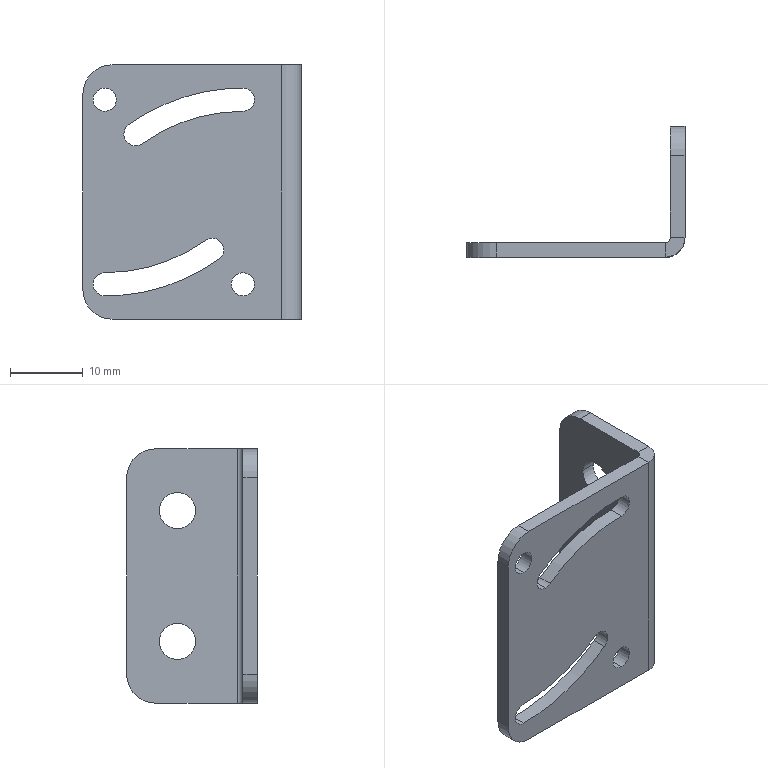Part | STEP file | KF-2212-070-006 | 1 solid | 35 faces | box 30 x 18 x 35 mm | volume 2796 mm3 | cylinder 23 | plane 12 | commonest cylinder face diameters 3.2 x9 5 x4 8 x4 47.6 x2 54 x2 1.473 x1
STEP:
#1=CARTESIAN_POINT('',(30.,6.5,-26.5));
#2=VERTEX_POINT('',#1);
#3=CARTESIAN_POINT('',(30.,11.5,-26.5));
#4=VERTEX_POINT('',#3);
#5=CARTESIAN_POINT('',(30.,9.,-26.5));
#6=DIRECTION('',(1.,0.,0.));
#7=DIRECTION('',(0.,-1.,0.));
#8=AXIS2_PLACEMENT_3D('',#5,#6,#7);
#9=CIRCLE('',#8,2.5);
#10=EDGE_CURVE('',#2,#4,#9,.T.);
#11=ORIENTED_EDGE('',*,*,#10,.T.);
#12=CARTESIAN_POINT('',(28.,11.5,-26.5));
#13=VERTEX_POINT('',#12);
#14=CARTESIAN_POINT('',(38.,11.5,-26.5));
#15=DIRECTION('',(-1.,0.,0.));
#16=VECTOR('',#15,1000.);
#17=LINE('',#14,#16);
#18=EDGE_CURVE('',#4,#13,#17,.T.);
#19=ORIENTED_EDGE('',*,*,#18,.T.);
#20=CARTESIAN_POINT('',(28.,6.5,-26.5));
#21=VERTEX_POINT('',#20);
#22=CARTESIAN_POINT('',(28.,9.,-26.5));
#23=DIRECTION('',(1.,0.,0.));
#24=DIRECTION('',(0.,-1.,0.));
#25=AXIS2_PLACEMENT_3D('',#22,#23,#24);
#26=CIRCLE('',#25,2.5);
#27=EDGE_CURVE('',#21,#13,#26,.T.);
#28=ORIENTED_EDGE('',*,*,#27,.F.);
#29=CARTESIAN_POINT('',(38.,6.5,-26.5));
#30=DIRECTION('',(-1.,0.,0.));
#31=VECTOR('',#30,1000.);
#32=LINE('',#29,#31);
#33=EDGE_CURVE('',#2,#21,#32,.T.);
#34=ORIENTED_EDGE('',*,*,#33,.F.);
#35=EDGE_LOOP('',(#11,#19,#28,#34));
#36=FACE_OUTER_BOUND('',#35,.T.);
#37=CARTESIAN_POINT('',(38.,9.,-26.5));
#38=DIRECTION('',(-1.,0.,0.));
#39=DIRECTION('',(0.,-1.,0.));
#40=AXIS2_PLACEMENT_3D('',#37,#38,#39);
#41=CYLINDRICAL_SURFACE('',#40,2.5);
#42=ADVANCED_FACE('',(#36),#41,.F.);
#43=CARTESIAN_POINT('',(30.,6.5,-8.5));
#44=VERTEX_POINT('',#43);
#45=CARTESIAN_POINT('',(30.,11.5,-8.5));
#46=VERTEX_POINT('',#45);
#47=CARTESIAN_POINT('',(30.,9.,-8.5));
#48=DIRECTION('',(1.,0.,0.));
#49=DIRECTION('',(0.,-1.,0.));
#50=AXIS2_PLACEMENT_3D('',#47,#48,#49);
#51=CIRCLE('',#50,2.5);
#52=EDGE_CURVE('',#44,#46,#51,.T.);
#53=ORIENTED_EDGE('',*,*,#52,.T.);
#54=CARTESIAN_POINT('',(28.,11.5,-8.5));
#55=VERTEX_POINT('',#54);
#56=CARTESIAN_POINT('',(38.,11.5,-8.5));
#57=DIRECTION('',(-1.,0.,0.));
#58=VECTOR('',#57,1000.);
#59=LINE('',#56,#58);
#60=EDGE_CURVE('',#46,#55,#59,.T.);
#61=ORIENTED_EDGE('',*,*,#60,.T.);
#62=CARTESIAN_POINT('',(28.,6.5,-8.5));
#63=VERTEX_POINT('',#62);
#64=CARTESIAN_POINT('',(28.,9.,-8.5));
#65=DIRECTION('',(1.,0.,0.));
#66=DIRECTION('',(0.,-1.,0.));
#67=AXIS2_PLACEMENT_3D('',#64,#65,#66);
#68=CIRCLE('',#67,2.5);
#69=EDGE_CURVE('',#63,#55,#68,.T.);
#70=ORIENTED_EDGE('',*,*,#69,.F.);
#71=CARTESIAN_POINT('',(38.,6.5,-8.5));
#72=DIRECTION('',(-1.,0.,0.));
#73=VECTOR('',#72,1000.);
#74=LINE('',#71,#73);
#75=EDGE_CURVE('',#44,#63,#74,.T.);
#76=ORIENTED_EDGE('',*,*,#75,.F.);
#77=EDGE_LOOP('',(#53,#61,#70,#76));
#78=FACE_OUTER_BOUND('',#77,.T.);
#79=CARTESIAN_POINT('',(38.,9.,-8.5));
#80=DIRECTION('',(-1.,0.,0.));
#81=DIRECTION('',(0.,-1.,0.));
#82=AXIS2_PLACEMENT_3D('',#79,#80,#81);
#83=CYLINDRICAL_SURFACE('',#82,2.5);
#84=ADVANCED_FACE('',(#78),#83,.F.);
#85=CARTESIAN_POINT('',(6.295,-2.,-8.237));
#86=VERTEX_POINT('',#85);
#87=CARTESIAN_POINT('',(7.226,-2.,-11.139));
#88=VERTEX_POINT('',#87);
#89=CARTESIAN_POINT('',(7.226,-2.,-9.539));
#90=DIRECTION('',(0.,-1.,0.));
#91=DIRECTION('',(0.,0.,-1.));
#92=AXIS2_PLACEMENT_3D('',#89,#90,#91);
#93=CIRCLE('',#92,1.6);
#94=EDGE_CURVE('',#86,#88,#93,.T.);
#95=ORIENTED_EDGE('',*,*,#94,.T.);
#96=CARTESIAN_POINT('',(7.226,0.,-11.139));
#97=VERTEX_POINT('',#96);
#98=CARTESIAN_POINT('',(7.226,-2.,-11.139));
#99=DIRECTION('',(0.,1.,0.));
#100=VECTOR('',#99,1000.);
#101=LINE('',#98,#100);
#102=EDGE_CURVE('',#88,#97,#101,.T.);
#103=ORIENTED_EDGE('',*,*,#102,.T.);
#104=CARTESIAN_POINT('',(6.295,0.,-8.237));
#105=VERTEX_POINT('',#104);
#106=CARTESIAN_POINT('',(7.226,0.,-9.539));
#107=DIRECTION('',(0.,-1.,0.));
#108=DIRECTION('',(0.,0.,-1.));
#109=AXIS2_PLACEMENT_3D('',#106,#107,#108);
#110=CIRCLE('',#109,1.6);
#111=EDGE_CURVE('',#105,#97,#110,.T.);
#112=ORIENTED_EDGE('',*,*,#111,.F.);
#113=CARTESIAN_POINT('',(6.295,-2.,-8.237));
#114=DIRECTION('',(0.,1.,0.));
#115=VECTOR('',#114,1000.);
#116=LINE('',#113,#115);
#117=EDGE_CURVE('',#86,#105,#116,.T.);
#118=ORIENTED_EDGE('',*,*,#117,.F.);
#119=EDGE_LOOP('',(#95,#103,#112,#118));
#120=FACE_OUTER_BOUND('',#119,.T.);
#121=CARTESIAN_POINT('',(7.226,-2.,-9.539));
#122=DIRECTION('',(0.,1.,0.));
#123=DIRECTION('',(0.,0.,-1.));
#124=AXIS2_PLACEMENT_3D('',#121,#122,#123);
#125=CYLINDRICAL_SURFACE('',#124,1.6);
#126=ADVANCED_FACE('',(#120),#125,.F.);
#127=CARTESIAN_POINT('',(22.,-2.,-31.8));
#128=VERTEX_POINT('',#127);
#129=CARTESIAN_POINT('',(22.,-2.,-28.6));
#130=VERTEX_POINT('',#129);
#131=CARTESIAN_POINT('',(22.,-2.,-30.2));
#132=DIRECTION('',(0.,-1.,0.));
#133=DIRECTION('',(0.,0.,-1.));
#134=AXIS2_PLACEMENT_3D('',#131,#132,#133);
#135=CIRCLE('',#134,1.6);
#136=EDGE_CURVE('',#128,#130,#135,.T.);
#137=ORIENTED_EDGE('',*,*,#136,.T.);
#138=CARTESIAN_POINT('',(22.,0.,-28.6));
#139=VERTEX_POINT('',#138);
#140=CARTESIAN_POINT('',(22.,-2.,-28.6));
#141=DIRECTION('',(0.,1.,0.));
#142=VECTOR('',#141,1000.);
#143=LINE('',#140,#142);
#144=EDGE_CURVE('',#130,#139,#143,.T.);
#145=ORIENTED_EDGE('',*,*,#144,.T.);
#146=CARTESIAN_POINT('',(22.,0.,-31.8));
#147=VERTEX_POINT('',#146);
#148=CARTESIAN_POINT('',(22.,0.,-30.2));
#149=DIRECTION('',(0.,-1.,0.));
#150=DIRECTION('',(0.,0.,-1.));
#151=AXIS2_PLACEMENT_3D('',#148,#149,#150);
#152=CIRCLE('',#151,1.6);
#153=EDGE_CURVE('',#147,#139,#152,.T.);
#154=ORIENTED_EDGE('',*,*,#153,.F.);
#155=CARTESIAN_POINT('',(22.,-2.,-31.8));
#156=DIRECTION('',(0.,1.,0.));
#157=VECTOR('',#156,1000.);
#158=LINE('',#155,#157);
#159=EDGE_CURVE('',#128,#147,#158,.T.);
#160=ORIENTED_EDGE('',*,*,#159,.F.);
#161=EDGE_LOOP('',(#137,#145,#154,#160));
#162=FACE_OUTER_BOUND('',#161,.T.);
#163=CARTESIAN_POINT('',(22.,-2.,-30.2));
#164=DIRECTION('',(0.,1.,0.));
#165=DIRECTION('',(0.,0.,-1.));
#166=AXIS2_PLACEMENT_3D('',#163,#164,#165);
#167=CYLINDRICAL_SURFACE('',#166,1.6);
#168=ADVANCED_FACE('',(#162),#167,.F.);
#169=CARTESIAN_POINT('',(3.,-2.,-6.4));
#170=VERTEX_POINT('',#169);
#171=CARTESIAN_POINT('',(3.,-2.,-3.2));
#172=VERTEX_POINT('',#171);
#173=CARTESIAN_POINT('',(3.,-2.,-4.8));
#174=DIRECTION('',(0.,-1.,0.));
#175=DIRECTION('',(0.,0.,-1.));
#176=AXIS2_PLACEMENT_3D('',#173,#174,#175);
#177=CIRCLE('',#176,1.6);
#178=EDGE_CURVE('',#170,#172,#177,.T.);
#179=ORIENTED_EDGE('',*,*,#178,.T.);
#180=CARTESIAN_POINT('',(3.,0.,-3.2));
#181=VERTEX_POINT('',#180);
#182=CARTESIAN_POINT('',(3.,-2.,-3.2));
#183=DIRECTION('',(0.,1.,0.));
#184=VECTOR('',#183,1000.);
#185=LINE('',#182,#184);
#186=EDGE_CURVE('',#172,#181,#185,.T.);
#187=ORIENTED_EDGE('',*,*,#186,.T.);
#188=CARTESIAN_POINT('',(3.,0.,-6.4));
#189=VERTEX_POINT('',#188);
#190=CARTESIAN_POINT('',(3.,0.,-4.8));
#191=DIRECTION('',(0.,-1.,0.));
#192=DIRECTION('',(0.,0.,-1.));
#193=AXIS2_PLACEMENT_3D('',#190,#191,#192);
#194=CIRCLE('',#193,1.6);
#195=EDGE_CURVE('',#189,#181,#194,.T.);
#196=ORIENTED_EDGE('',*,*,#195,.F.);
#197=CARTESIAN_POINT('',(3.,-2.,-6.4));
#198=DIRECTION('',(0.,1.,0.));
#199=VECTOR('',#198,1000.);
#200=LINE('',#197,#199);
#201=EDGE_CURVE('',#170,#189,#200,.T.);
#202=ORIENTED_EDGE('',*,*,#201,.F.);
#203=EDGE_LOOP('',(#179,#187,#196,#202));
#204=FACE_OUTER_BOUND('',#203,.T.);
#205=CARTESIAN_POINT('',(3.,-2.,-4.8));
#206=DIRECTION('',(0.,1.,0.));
#207=DIRECTION('',(0.,0.,-1.));
#208=AXIS2_PLACEMENT_3D('',#205,#206,#207);
#209=CYLINDRICAL_SURFACE('',#208,1.6);
#210=ADVANCED_FACE('',(#204),#209,.F.);
#211=CARTESIAN_POINT('',(27.263,-2.,0.));
#212=VERTEX_POINT('',#211);
#213=CARTESIAN_POINT('',(4.,-2.,0.));
#214=VERTEX_POINT('',#213);
#215=CARTESIAN_POINT('',(0.,-2.,0.));
#216=DIRECTION('',(-1.,0.,0.));
#217=VECTOR('',#216,1000.);
#218=LINE('',#215,#217);
#219=EDGE_CURVE('',#212,#214,#218,.T.);
#220=ORIENTED_EDGE('',*,*,#219,.F.);
#221=CARTESIAN_POINT('',(27.263,0.,0.));
#222=VERTEX_POINT('',#221);
#223=CARTESIAN_POINT('',(27.263,0.,0.));
#224=DIRECTION('',(0.,-1.,0.));
#225=VECTOR('',#224,1000.);
#226=LINE('',#223,#225);
#227=EDGE_CURVE('',#222,#212,#226,.T.);
#228=ORIENTED_EDGE('',*,*,#227,.F.);
#229=CARTESIAN_POINT('',(4.,0.,0.));
#230=VERTEX_POINT('',#229);
#231=CARTESIAN_POINT('',(0.,0.,0.));
#232=DIRECTION('',(-1.,0.,0.));
#233=VECTOR('',#232,1000.);
#234=LINE('',#231,#233);
#235=EDGE_CURVE('',#222,#230,#234,.T.);
#236=ORIENTED_EDGE('',*,*,#235,.T.);
#237=CARTESIAN_POINT('',(4.,-2.,0.));
#238=DIRECTION('',(0.,1.,0.));
#239=VECTOR('',#238,1000.);
#240=LINE('',#237,#239);
#241=EDGE_CURVE('',#214,#230,#240,.T.);
#242=ORIENTED_EDGE('',*,*,#241,.F.);
#243=EDGE_LOOP('',(#220,#228,#236,#242));
#244=FACE_OUTER_BOUND('',#243,.T.);
#245=CARTESIAN_POINT('',(0.,-2.,0.));
#246=DIRECTION('',(0.,0.,1.));
#247=DIRECTION('',(-1.,0.,0.));
#248=AXIS2_PLACEMENT_3D('',#245,#246,#247);
#249=PLANE('',#248);
#250=ADVANCED_FACE('',(#244),#249,.T.);
#251=CARTESIAN_POINT('',(8.156,-2.,-10.84));
#252=VERTEX_POINT('',#251);
#253=CARTESIAN_POINT('',(22.,-2.,-6.4));
#254=VERTEX_POINT('',#253);
#255=CARTESIAN_POINT('',(22.,-2.,-30.2));
#256=DIRECTION('',(0.,1.,0.));
#257=DIRECTION('',(0.,0.,-1.));
#258=AXIS2_PLACEMENT_3D('',#255,#256,#257);
#259=CIRCLE('',#258,23.8);
#260=EDGE_CURVE('',#252,#254,#259,.T.);
#261=ORIENTED_EDGE('',*,*,#260,.F.);
#262=CARTESIAN_POINT('',(7.226,-2.,-9.539));
#263=DIRECTION('',(0.,-1.,0.));
#264=DIRECTION('',(0.,0.,-1.));
#265=AXIS2_PLACEMENT_3D('',#262,#263,#264);
#266=CIRCLE('',#265,1.6);
#267=EDGE_CURVE('',#88,#252,#266,.T.);
#268=ORIENTED_EDGE('',*,*,#267,.F.);
#269=ORIENTED_EDGE('',*,*,#94,.F.);
#270=CARTESIAN_POINT('',(22.,-2.,-3.2));
#271=VERTEX_POINT('',#270);
#272=CARTESIAN_POINT('',(22.,-2.,-30.2));
#273=DIRECTION('',(0.,-1.,0.));
#274=DIRECTION('',(0.,0.,-1.));
#275=AXIS2_PLACEMENT_3D('',#272,#273,#274);
#276=CIRCLE('',#275,27.);
#277=EDGE_CURVE('',#271,#86,#276,.T.);
#278=ORIENTED_EDGE('',*,*,#277,.F.);
#279=CARTESIAN_POINT('',(22.,-2.,-4.8));
#280=DIRECTION('',(0.,-1.,0.));
#281=DIRECTION('',(0.,0.,-1.));
#282=AXIS2_PLACEMENT_3D('',#279,#280,#281);
#283=CIRCLE('',#282,1.6);
#284=EDGE_CURVE('',#254,#271,#283,.T.);
#285=ORIENTED_EDGE('',*,*,#284,.F.);
#286=EDGE_LOOP('',(#261,#268,#269,#278,#285));
#287=FACE_BOUND('',#286,.T.);
#288=CARTESIAN_POINT('',(3.,-2.,-28.6));
#289=VERTEX_POINT('',#288);
#290=CARTESIAN_POINT('',(3.,-2.,-31.8));
#291=VERTEX_POINT('',#290);
#292=CARTESIAN_POINT('',(3.,-2.,-30.2));
#293=DIRECTION('',(0.,-1.,0.));
#294=DIRECTION('',(0.,0.,-1.));
#295=AXIS2_PLACEMENT_3D('',#292,#293,#294);
#296=CIRCLE('',#295,1.6);
#297=EDGE_CURVE('',#289,#291,#296,.T.);
#298=ORIENTED_EDGE('',*,*,#297,.F.);
#299=CARTESIAN_POINT('',(16.844,-2.,-24.16));
#300=VERTEX_POINT('',#299);
#301=CARTESIAN_POINT('',(3.,-2.,-4.8));
#302=DIRECTION('',(0.,1.,0.));
#303=DIRECTION('',(0.,0.,-1.));
#304=AXIS2_PLACEMENT_3D('',#301,#302,#303);
#305=CIRCLE('',#304,23.8);
#306=EDGE_CURVE('',#300,#289,#305,.T.);
#307=ORIENTED_EDGE('',*,*,#306,.F.);
#308=CARTESIAN_POINT('',(18.705,-2.,-26.763));
#309=VERTEX_POINT('',#308);
#310=CARTESIAN_POINT('',(17.774,-2.,-25.461));
#311=DIRECTION('',(0.,-1.,0.));
#312=DIRECTION('',(0.,0.,-1.));
#313=AXIS2_PLACEMENT_3D('',#310,#311,#312);
#314=CIRCLE('',#313,1.6);
#315=EDGE_CURVE('',#309,#300,#314,.T.);
#316=ORIENTED_EDGE('',*,*,#315,.F.);
#317=CARTESIAN_POINT('',(3.,-2.,-4.8));
#318=DIRECTION('',(0.,-1.,0.));
#319=DIRECTION('',(0.,0.,-1.));
#320=AXIS2_PLACEMENT_3D('',#317,#318,#319);
#321=CIRCLE('',#320,27.);
#322=EDGE_CURVE('',#291,#309,#321,.T.);
#323=ORIENTED_EDGE('',*,*,#322,.F.);
#324=EDGE_LOOP('',(#298,#307,#316,#323));
#325=FACE_BOUND('',#324,.T.);
#326=ORIENTED_EDGE('',*,*,#136,.F.);
#327=CARTESIAN_POINT('',(22.,-2.,-30.2));
#328=DIRECTION('',(0.,-1.,0.));
#329=DIRECTION('',(0.,0.,-1.));
#330=AXIS2_PLACEMENT_3D('',#327,#328,#329);
#331=CIRCLE('',#330,1.6);
#332=EDGE_CURVE('',#130,#128,#331,.T.);
#333=ORIENTED_EDGE('',*,*,#332,.F.);
#334=EDGE_LOOP('',(#326,#333));
#335=FACE_BOUND('',#334,.T.);
#336=ORIENTED_EDGE('',*,*,#178,.F.);
#337=CARTESIAN_POINT('',(3.,-2.,-4.8));
#338=DIRECTION('',(0.,-1.,0.));
#339=DIRECTION('',(0.,0.,-1.));
#340=AXIS2_PLACEMENT_3D('',#337,#338,#339);
#341=CIRCLE('',#340,1.6);
#342=EDGE_CURVE('',#172,#170,#341,.T.);
#343=ORIENTED_EDGE('',*,*,#342,.F.);
#344=EDGE_LOOP('',(#336,#343));
#345=FACE_BOUND('',#344,.T.);
#346=CARTESIAN_POINT('',(0.,-2.,-4.));
#347=VERTEX_POINT('',#346);
#348=CARTESIAN_POINT('',(0.,-2.,-31.));
#349=VERTEX_POINT('',#348);
#350=CARTESIAN_POINT('',(0.,-2.,0.));
#351=DIRECTION('',(0.,0.,-1.));
#352=VECTOR('',#351,1000.);
#353=LINE('',#350,#352);
#354=EDGE_CURVE('',#347,#349,#353,.T.);
#355=ORIENTED_EDGE('',*,*,#354,.T.);
#356=CARTESIAN_POINT('',(4.,-2.,-35.));
#357=VERTEX_POINT('',#356);
#358=CARTESIAN_POINT('',(4.,-2.,-31.));
#359=DIRECTION('',(0.,1.,0.));
#360=DIRECTION('',(0.,0.,-1.));
#361=AXIS2_PLACEMENT_3D('',#358,#359,#360);
#362=CIRCLE('',#361,4.);
#363=EDGE_CURVE('',#357,#349,#362,.T.);
#364=ORIENTED_EDGE('',*,*,#363,.F.);
#365=CARTESIAN_POINT('',(27.263,-2.,-35.));
#366=VERTEX_POINT('',#365);
#367=CARTESIAN_POINT('',(0.,-2.,-35.));
#368=DIRECTION('',(1.,0.,0.));
#369=VECTOR('',#368,1000.);
#370=LINE('',#367,#369);
#371=EDGE_CURVE('',#357,#366,#370,.T.);
#372=ORIENTED_EDGE('',*,*,#371,.T.);
#373=CARTESIAN_POINT('',(27.263,-2.,0.));
#374=DIRECTION('',(0.,0.,-1.));
#375=VECTOR('',#374,1000.);
#376=LINE('',#373,#375);
#377=EDGE_CURVE('',#212,#366,#376,.T.);
#378=ORIENTED_EDGE('',*,*,#377,.F.);
#379=ORIENTED_EDGE('',*,*,#219,.T.);
#380=CARTESIAN_POINT('',(4.,-2.,-4.));
#381=DIRECTION('',(0.,1.,0.));
#382=DIRECTION('',(0.,0.,-1.));
#383=AXIS2_PLACEMENT_3D('',#380,#381,#382);
#384=CIRCLE('',#383,4.);
#385=EDGE_CURVE('',#347,#214,#384,.T.);
#386=ORIENTED_EDGE('',*,*,#385,.F.);
#387=EDGE_LOOP('',(#355,#364,#372,#378,#379,#386));
#388=FACE_OUTER_BOUND('',#387,.T.);
#389=CARTESIAN_POINT('',(0.,-2.,0.));
#390=DIRECTION('',(0.,1.,0.));
#391=DIRECTION('',(0.,0.,-1.));
#392=AXIS2_PLACEMENT_3D('',#389,#390,#391);
#393=PLANE('',#392);
#394=ADVANCED_FACE('',(#287,#325,#335,#345,#388),#393,.F.);
#395=CARTESIAN_POINT('',(22.,0.,-6.4));
#396=VERTEX_POINT('',#395);
#397=CARTESIAN_POINT('',(22.,0.,-3.2));
#398=VERTEX_POINT('',#397);
#399=CARTESIAN_POINT('',(22.,0.,-4.8));
#400=DIRECTION('',(0.,-1.,0.));
#401=DIRECTION('',(0.,0.,-1.));
#402=AXIS2_PLACEMENT_3D('',#399,#400,#401);
#403=CIRCLE('',#402,1.6);
#404=EDGE_CURVE('',#396,#398,#403,.T.);
#405=ORIENTED_EDGE('',*,*,#404,.T.);
#406=CARTESIAN_POINT('',(22.,0.,-30.2));
#407=DIRECTION('',(0.,-1.,0.));
#408=DIRECTION('',(0.,0.,-1.));
#409=AXIS2_PLACEMENT_3D('',#406,#407,#408);
#410=CIRCLE('',#409,27.);
#411=EDGE_CURVE('',#398,#105,#410,.T.);
#412=ORIENTED_EDGE('',*,*,#411,.T.);
#413=ORIENTED_EDGE('',*,*,#111,.T.);
#414=CARTESIAN_POINT('',(8.156,0.,-10.84));
#415=VERTEX_POINT('',#414);
#416=CARTESIAN_POINT('',(7.226,0.,-9.539));
#417=DIRECTION('',(0.,-1.,0.));
#418=DIRECTION('',(0.,0.,-1.));
#419=AXIS2_PLACEMENT_3D('',#416,#417,#418);
#420=CIRCLE('',#419,1.6);
#421=EDGE_CURVE('',#97,#415,#420,.T.);
#422=ORIENTED_EDGE('',*,*,#421,.T.);
#423=CARTESIAN_POINT('',(22.,0.,-30.2));
#424=DIRECTION('',(0.,1.,0.));
#425=DIRECTION('',(0.,0.,-1.));
#426=AXIS2_PLACEMENT_3D('',#423,#424,#425);
#427=CIRCLE('',#426,23.8);
#428=EDGE_CURVE('',#415,#396,#427,.T.);
#429=ORIENTED_EDGE('',*,*,#428,.T.);
#430=EDGE_LOOP('',(#405,#412,#413,#422,#429));
#431=FACE_BOUND('',#430,.T.);
#432=CARTESIAN_POINT('',(3.,0.,-31.8));
#433=VERTEX_POINT('',#432);
#434=CARTESIAN_POINT('',(18.705,0.,-26.763));
#435=VERTEX_POINT('',#434);
#436=CARTESIAN_POINT('',(3.,0.,-4.8));
#437=DIRECTION('',(0.,-1.,0.));
#438=DIRECTION('',(0.,0.,-1.));
#439=AXIS2_PLACEMENT_3D('',#436,#437,#438);
#440=CIRCLE('',#439,27.);
#441=EDGE_CURVE('',#433,#435,#440,.T.);
#442=ORIENTED_EDGE('',*,*,#441,.T.);
#443=CARTESIAN_POINT('',(16.844,0.,-24.16));
#444=VERTEX_POINT('',#443);
#445=CARTESIAN_POINT('',(17.774,0.,-25.461));
#446=DIRECTION('',(0.,-1.,0.));
#447=DIRECTION('',(0.,0.,-1.));
#448=AXIS2_PLACEMENT_3D('',#445,#446,#447);
#449=CIRCLE('',#448,1.6);
#450=EDGE_CURVE('',#435,#444,#449,.T.);
#451=ORIENTED_EDGE('',*,*,#450,.T.);
#452=CARTESIAN_POINT('',(3.,0.,-28.6));
#453=VERTEX_POINT('',#452);
#454=CARTESIAN_POINT('',(3.,0.,-4.8));
#455=DIRECTION('',(0.,1.,0.));
#456=DIRECTION('',(0.,0.,-1.));
#457=AXIS2_PLACEMENT_3D('',#454,#455,#456);
#458=CIRCLE('',#457,23.8);
#459=EDGE_CURVE('',#444,#453,#458,.T.);
#460=ORIENTED_EDGE('',*,*,#459,.T.);
#461=CARTESIAN_POINT('',(3.,0.,-30.2));
#462=DIRECTION('',(0.,-1.,0.));
#463=DIRECTION('',(0.,0.,-1.));
#464=AXIS2_PLACEMENT_3D('',#461,#462,#463);
#465=CIRCLE('',#464,1.6);
#466=EDGE_CURVE('',#453,#433,#465,.T.);
#467=ORIENTED_EDGE('',*,*,#466,.T.);
#468=EDGE_LOOP('',(#442,#451,#460,#467));
#469=FACE_BOUND('',#468,.T.);
#470=ORIENTED_EDGE('',*,*,#153,.T.);
#471=CARTESIAN_POINT('',(22.,0.,-30.2));
#472=DIRECTION('',(0.,-1.,0.));
#473=DIRECTION('',(0.,0.,-1.));
#474=AXIS2_PLACEMENT_3D('',#471,#472,#473);
#475=CIRCLE('',#474,1.6);
#476=EDGE_CURVE('',#139,#147,#475,.T.);
#477=ORIENTED_EDGE('',*,*,#476,.T.);
#478=EDGE_LOOP('',(#470,#477));
#479=FACE_BOUND('',#478,.T.);
#480=ORIENTED_EDGE('',*,*,#195,.T.);
#481=CARTESIAN_POINT('',(3.,0.,-4.8));
#482=DIRECTION('',(0.,-1.,0.));
#483=DIRECTION('',(0.,0.,-1.));
#484=AXIS2_PLACEMENT_3D('',#481,#482,#483);
#485=CIRCLE('',#484,1.6);
#486=EDGE_CURVE('',#181,#189,#485,.T.);
#487=ORIENTED_EDGE('',*,*,#486,.T.);
#488=EDGE_LOOP('',(#480,#487));
#489=FACE_BOUND('',#488,.T.);
#490=ORIENTED_EDGE('',*,*,#235,.F.);
#491=CARTESIAN_POINT('',(27.263,0.,-35.));
#492=VERTEX_POINT('',#491);
#493=CARTESIAN_POINT('',(27.263,0.,0.));
#494=DIRECTION('',(0.,0.,-1.));
#495=VECTOR('',#494,1000.);
#496=LINE('',#493,#495);
#497=EDGE_CURVE('',#222,#492,#496,.T.);
#498=ORIENTED_EDGE('',*,*,#497,.T.);
#499=CARTESIAN_POINT('',(4.,0.,-35.));
#500=VERTEX_POINT('',#499);
#501=CARTESIAN_POINT('',(0.,0.,-35.));
#502=DIRECTION('',(1.,0.,0.));
#503=VECTOR('',#502,1000.);
#504=LINE('',#501,#503);
#505=EDGE_CURVE('',#500,#492,#504,.T.);
#506=ORIENTED_EDGE('',*,*,#505,.F.);
#507=CARTESIAN_POINT('',(0.,0.,-31.));
#508=VERTEX_POINT('',#507);
#509=CARTESIAN_POINT('',(4.,0.,-31.));
#510=DIRECTION('',(0.,-1.,0.));
#511=DIRECTION('',(0.,0.,-1.));
#512=AXIS2_PLACEMENT_3D('',#509,#510,#511);
#513=CIRCLE('',#512,4.);
#514=EDGE_CURVE('',#508,#500,#513,.T.);
#515=ORIENTED_EDGE('',*,*,#514,.F.);
#516=CARTESIAN_POINT('',(0.,0.,-4.));
#517=VERTEX_POINT('',#516);
#518=CARTESIAN_POINT('',(0.,0.,0.));
#519=DIRECTION('',(0.,0.,-1.));
#520=VECTOR('',#519,1000.);
#521=LINE('',#518,#520);
#522=EDGE_CURVE('',#517,#508,#521,.T.);
#523=ORIENTED_EDGE('',*,*,#522,.F.);
#524=CARTESIAN_POINT('',(4.,0.,-4.));
#525=DIRECTION('',(0.,-1.,0.));
#526=DIRECTION('',(0.,0.,-1.));
#527=AXIS2_PLACEMENT_3D('',#524,#525,#526);
#528=CIRCLE('',#527,4.);
#529=EDGE_CURVE('',#230,#517,#528,.T.);
#530=ORIENTED_EDGE('',*,*,#529,.F.);
#531=EDGE_LOOP('',(#490,#498,#506,#515,#523,#530));
#532=FACE_OUTER_BOUND('',#531,.T.);
#533=CARTESIAN_POINT('',(0.,0.,0.));
#534=DIRECTION('',(0.,1.,0.));
#535=DIRECTION('',(0.,0.,-1.));
#536=AXIS2_PLACEMENT_3D('',#533,#534,#535);
#537=PLANE('',#536);
#538=ADVANCED_FACE('',(#431,#469,#479,#489,#532),#537,.T.);
#539=ORIENTED_EDGE('',*,*,#522,.T.);
#540=CARTESIAN_POINT('',(0.,-2.,-31.));
#541=DIRECTION('',(0.,1.,0.));
#542=VECTOR('',#541,1000.);
#543=LINE('',#540,#542);
#544=EDGE_CURVE('',#349,#508,#543,.T.);
#545=ORIENTED_EDGE('',*,*,#544,.F.);
#546=ORIENTED_EDGE('',*,*,#354,.F.);
#547=CARTESIAN_POINT('',(0.,-2.,-4.));
#548=DIRECTION('',(0.,-1.,0.));
#549=VECTOR('',#548,1000.);
#550=LINE('',#547,#549);
#551=EDGE_CURVE('',#517,#347,#550,.T.);
#552=ORIENTED_EDGE('',*,*,#551,.F.);
#553=EDGE_LOOP('',(#539,#545,#546,#552));
#554=FACE_OUTER_BOUND('',#553,.T.);
#555=CARTESIAN_POINT('',(0.,-2.,0.));
#556=DIRECTION('',(-1.,0.,0.));
#557=DIRECTION('',(0.,0.,-1.));
#558=AXIS2_PLACEMENT_3D('',#555,#556,#557);
#559=PLANE('',#558);
#560=ADVANCED_FACE('',(#554),#559,.T.);
#561=ORIENTED_EDGE('',*,*,#505,.T.);
#562=CARTESIAN_POINT('',(27.263,0.,-35.));
#563=DIRECTION('',(0.,-1.,0.));
#564=VECTOR('',#563,1000.);
#565=LINE('',#562,#564);
#566=EDGE_CURVE('',#492,#366,#565,.T.);
#567=ORIENTED_EDGE('',*,*,#566,.T.);
#568=ORIENTED_EDGE('',*,*,#371,.F.);
#569=CARTESIAN_POINT('',(4.,-2.,-35.));
#570=DIRECTION('',(0.,-1.,0.));
#571=VECTOR('',#570,1000.);
#572=LINE('',#569,#571);
#573=EDGE_CURVE('',#500,#357,#572,.T.);
#574=ORIENTED_EDGE('',*,*,#573,.F.);
#575=EDGE_LOOP('',(#561,#567,#568,#574));
#576=FACE_OUTER_BOUND('',#575,.T.);
#577=CARTESIAN_POINT('',(0.,-2.,-35.));
#578=DIRECTION('',(0.,0.,-1.));
#579=DIRECTION('',(1.,0.,0.));
#580=AXIS2_PLACEMENT_3D('',#577,#578,#579);
#581=PLANE('',#580);
#582=ADVANCED_FACE('',(#576),#581,.T.);
#583=CARTESIAN_POINT('',(28.,0.7366,-35.));
#584=VERTEX_POINT('',#583);
#585=CARTESIAN_POINT('',(30.,0.7366,-35.));
#586=VERTEX_POINT('',#585);
#587=CARTESIAN_POINT('',(30.,0.7366,-35.));
#588=DIRECTION('',(1.,0.,0.));
#589=VECTOR('',#588,1000.);
#590=LINE('',#587,#589);
#591=EDGE_CURVE('',#584,#586,#590,.T.);
#592=ORIENTED_EDGE('',*,*,#591,.T.);
#593=CARTESIAN_POINT('',(27.263,0.7366,-35.));
#594=DIRECTION('',(0.,0.,1.));
#595=DIRECTION('',(0.,1.,0.));
#596=AXIS2_PLACEMENT_3D('',#593,#594,#595);
#597=CIRCLE('',#596,2.737);
#598=EDGE_CURVE('',#366,#586,#597,.T.);
#599=ORIENTED_EDGE('',*,*,#598,.F.);
#600=ORIENTED_EDGE('',*,*,#566,.F.);
#601=CARTESIAN_POINT('',(27.263,0.7366,-35.));
#602=DIRECTION('',(0.,0.,1.));
#603=DIRECTION('',(0.,1.,0.));
#604=AXIS2_PLACEMENT_3D('',#601,#602,#603);
#605=CIRCLE('',#604,0.7366);
#606=EDGE_CURVE('',#492,#584,#605,.T.);
#607=ORIENTED_EDGE('',*,*,#606,.T.);
#608=EDGE_LOOP('',(#592,#599,#600,#607));
#609=FACE_OUTER_BOUND('',#608,.T.);
#610=CARTESIAN_POINT('',(27.263,0.7366,-35.));
#611=DIRECTION('',(0.,0.,-1.));
#612=DIRECTION('',(0.,-1.,0.));
#613=AXIS2_PLACEMENT_3D('',#610,#611,#612);
#614=PLANE('',#613);
#615=ADVANCED_FACE('',(#609),#614,.T.);
#616=CARTESIAN_POINT('',(28.,0.7366,0.));
#617=VERTEX_POINT('',#616);
#618=CARTESIAN_POINT('',(27.263,0.7366,0.));
#619=DIRECTION('',(0.,0.,-1.));
#620=DIRECTION('',(0.,1.,0.));
#621=AXIS2_PLACEMENT_3D('',#618,#619,#620);
#622=CIRCLE('',#621,0.7366);
#623=EDGE_CURVE('',#617,#222,#622,.T.);
#624=ORIENTED_EDGE('',*,*,#623,.T.);
#625=ORIENTED_EDGE('',*,*,#227,.T.);
#626=CARTESIAN_POINT('',(30.,0.7366,0.));
#627=VERTEX_POINT('',#626);
#628=CARTESIAN_POINT('',(27.263,0.7366,0.));
#629=DIRECTION('',(0.,0.,-1.));
#630=DIRECTION('',(0.,1.,0.));
#631=AXIS2_PLACEMENT_3D('',#628,#629,#630);
#632=CIRCLE('',#631,2.737);
#633=EDGE_CURVE('',#627,#212,#632,.T.);
#634=ORIENTED_EDGE('',*,*,#633,.F.);
#635=CARTESIAN_POINT('',(28.,0.7366,0.));
#636=DIRECTION('',(1.,0.,0.));
#637=VECTOR('',#636,1000.);
#638=LINE('',#635,#637);
#639=EDGE_CURVE('',#617,#627,#638,.T.);
#640=ORIENTED_EDGE('',*,*,#639,.F.);
#641=EDGE_LOOP('',(#624,#625,#634,#640));
#642=FACE_OUTER_BOUND('',#641,.T.);
#643=CARTESIAN_POINT('',(27.263,0.7366,0.));
#644=DIRECTION('',(0.,0.,-1.));
#645=DIRECTION('',(0.,-1.,0.));
#646=AXIS2_PLACEMENT_3D('',#643,#644,#645);
#647=PLANE('',#646);
#648=ADVANCED_FACE('',(#642),#647,.F.);
#649=ORIENTED_EDGE('',*,*,#377,.T.);
#650=ORIENTED_EDGE('',*,*,#598,.T.);
#651=CARTESIAN_POINT('',(30.,0.7366,-35.));
#652=DIRECTION('',(0.,0.,-1.));
#653=VECTOR('',#652,1000.);
#654=LINE('',#651,#653);
#655=EDGE_CURVE('',#627,#586,#654,.T.);
#656=ORIENTED_EDGE('',*,*,#655,.F.);
#657=ORIENTED_EDGE('',*,*,#633,.T.);
#658=EDGE_LOOP('',(#649,#650,#656,#657));
#659=FACE_OUTER_BOUND('',#658,.T.);
#660=CARTESIAN_POINT('',(27.263,0.7366,0.));
#661=DIRECTION('',(0.,0.,1.));
#662=DIRECTION('',(1.,0.,0.));
#663=AXIS2_PLACEMENT_3D('',#660,#661,#662);
#664=CYLINDRICAL_SURFACE('',#663,2.737);
#665=ADVANCED_FACE('',(#659),#664,.T.);
#666=ORIENTED_EDGE('',*,*,#497,.F.);
#667=ORIENTED_EDGE('',*,*,#623,.F.);
#668=CARTESIAN_POINT('',(28.,0.7366,-35.));
#669=DIRECTION('',(0.,0.,1.));
#670=VECTOR('',#669,1000.);
#671=LINE('',#668,#670);
#672=EDGE_CURVE('',#584,#617,#671,.T.);
#673=ORIENTED_EDGE('',*,*,#672,.F.);
#674=ORIENTED_EDGE('',*,*,#606,.F.);
#675=EDGE_LOOP('',(#666,#667,#673,#674));
#676=FACE_OUTER_BOUND('',#675,.T.);
#677=CARTESIAN_POINT('',(27.263,0.7366,0.));
#678=DIRECTION('',(0.,0.,1.));
#679=DIRECTION('',(1.,0.,0.));
#680=AXIS2_PLACEMENT_3D('',#677,#678,#679);
#681=CYLINDRICAL_SURFACE('',#680,0.7366);
#682=ADVANCED_FACE('',(#676),#681,.F.);
#683=CARTESIAN_POINT('',(30.,12.,-35.));
#684=VERTEX_POINT('',#683);
#685=CARTESIAN_POINT('',(30.,0.,-35.));
#686=DIRECTION('',(0.,-1.,0.));
#687=VECTOR('',#686,1000.);
#688=LINE('',#685,#687);
#689=EDGE_CURVE('',#684,#586,#688,.T.);
#690=ORIENTED_EDGE('',*,*,#689,.T.);
#691=ORIENTED_EDGE('',*,*,#591,.F.);
#692=CARTESIAN_POINT('',(28.,12.,-35.));
#693=VERTEX_POINT('',#692);
#694=CARTESIAN_POINT('',(28.,0.,-35.));
#695=DIRECTION('',(0.,-1.,0.));
#696=VECTOR('',#695,1000.);
#697=LINE('',#694,#696);
#698=EDGE_CURVE('',#693,#584,#697,.T.);
#699=ORIENTED_EDGE('',*,*,#698,.F.);
#700=CARTESIAN_POINT('',(30.,12.,-35.));
#701=DIRECTION('',(-1.,0.,0.));
#702=VECTOR('',#701,1000.);
#703=LINE('',#700,#702);
#704=EDGE_CURVE('',#684,#693,#703,.T.);
#705=ORIENTED_EDGE('',*,*,#704,.F.);
#706=EDGE_LOOP('',(#690,#691,#699,#705));
#707=FACE_OUTER_BOUND('',#706,.T.);
#708=CARTESIAN_POINT('',(30.,0.,-35.));
#709=DIRECTION('',(0.,0.,1.));
#710=DIRECTION('',(-1.,0.,0.));
#711=AXIS2_PLACEMENT_3D('',#708,#709,#710);
#712=PLANE('',#711);
#713=ADVANCED_FACE('',(#707),#712,.F.);
#714=CARTESIAN_POINT('',(28.,12.,0.));
#715=VERTEX_POINT('',#714);
#716=CARTESIAN_POINT('',(28.,16.,0.));
#717=DIRECTION('',(0.,1.,0.));
#718=VECTOR('',#717,1000.);
#719=LINE('',#716,#718);
#720=EDGE_CURVE('',#617,#715,#719,.T.);
#721=ORIENTED_EDGE('',*,*,#720,.F.);
#722=ORIENTED_EDGE('',*,*,#639,.T.);
#723=CARTESIAN_POINT('',(30.,12.,0.));
#724=VERTEX_POINT('',#723);
#725=CARTESIAN_POINT('',(30.,0.,0.));
#726=DIRECTION('',(0.,1.,0.));
#727=VECTOR('',#726,1000.);
#728=LINE('',#725,#727);
#729=EDGE_CURVE('',#627,#724,#728,.T.);
#730=ORIENTED_EDGE('',*,*,#729,.T.);
#731=CARTESIAN_POINT('',(30.,12.,0.));
#732=DIRECTION('',(1.,0.,0.));
#733=VECTOR('',#732,1000.);
#734=LINE('',#731,#733);
#735=EDGE_CURVE('',#715,#724,#734,.T.);
#736=ORIENTED_EDGE('',*,*,#735,.F.);
#737=EDGE_LOOP('',(#721,#722,#730,#736));
#738=FACE_OUTER_BOUND('',#737,.T.);
#739=CARTESIAN_POINT('',(30.,16.,0.));
#740=DIRECTION('',(0.,0.,-1.));
#741=DIRECTION('',(0.,-1.,0.));
#742=AXIS2_PLACEMENT_3D('',#739,#740,#741);
#743=PLANE('',#742);
#744=ADVANCED_FACE('',(#738),#743,.F.);
#745=ORIENTED_EDGE('',*,*,#10,.F.);
#746=CARTESIAN_POINT('',(30.,9.,-26.5));
#747=DIRECTION('',(1.,0.,0.));
#748=DIRECTION('',(0.,-1.,0.));
#749=AXIS2_PLACEMENT_3D('',#746,#747,#748);
#750=CIRCLE('',#749,2.5);
#751=EDGE_CURVE('',#4,#2,#750,.T.);
#752=ORIENTED_EDGE('',*,*,#751,.F.);
#753=EDGE_LOOP('',(#745,#752));
#754=FACE_BOUND('',#753,.T.);
#755=ORIENTED_EDGE('',*,*,#52,.F.);
#756=CARTESIAN_POINT('',(30.,9.,-8.5));
#757=DIRECTION('',(1.,0.,0.));
#758=DIRECTION('',(0.,-1.,0.));
#759=AXIS2_PLACEMENT_3D('',#756,#757,#758);
#760=CIRCLE('',#759,2.5);
#761=EDGE_CURVE('',#46,#44,#760,.T.);
#762=ORIENTED_EDGE('',*,*,#761,.F.);
#763=EDGE_LOOP('',(#755,#762));
#764=FACE_BOUND('',#763,.T.);
#765=ORIENTED_EDGE('',*,*,#729,.F.);
#766=ORIENTED_EDGE('',*,*,#655,.T.);
#767=ORIENTED_EDGE('',*,*,#689,.F.);
#768=CARTESIAN_POINT('',(30.,16.,-31.));
#769=VERTEX_POINT('',#768);
#770=CARTESIAN_POINT('',(30.,12.,-31.));
#771=DIRECTION('',(-1.,0.,0.));
#772=DIRECTION('',(0.,-1.,0.));
#773=AXIS2_PLACEMENT_3D('',#770,#771,#772);
#774=CIRCLE('',#773,4.);
#775=EDGE_CURVE('',#769,#684,#774,.T.);
#776=ORIENTED_EDGE('',*,*,#775,.F.);
#777=CARTESIAN_POINT('',(30.,16.,-4.));
#778=VERTEX_POINT('',#777);
#779=CARTESIAN_POINT('',(30.,16.,0.));
#780=DIRECTION('',(0.,0.,-1.));
#781=VECTOR('',#780,1000.);
#782=LINE('',#779,#781);
#783=EDGE_CURVE('',#778,#769,#782,.T.);
#784=ORIENTED_EDGE('',*,*,#783,.F.);
#785=CARTESIAN_POINT('',(30.,12.,-4.));
#786=DIRECTION('',(-1.,0.,0.));
#787=DIRECTION('',(0.,-1.,0.));
#788=AXIS2_PLACEMENT_3D('',#785,#786,#787);
#789=CIRCLE('',#788,4.);
#790=EDGE_CURVE('',#724,#778,#789,.T.);
#791=ORIENTED_EDGE('',*,*,#790,.F.);
#792=EDGE_LOOP('',(#765,#766,#767,#776,#784,#791));
#793=FACE_OUTER_BOUND('',#792,.T.);
#794=CARTESIAN_POINT('',(30.,0.,0.));
#795=DIRECTION('',(-1.,0.,0.));
#796=DIRECTION('',(0.,-1.,0.));
#797=AXIS2_PLACEMENT_3D('',#794,#795,#796);
#798=PLANE('',#797);
#799=ADVANCED_FACE('',(#754,#764,#793),#798,.F.);
#800=ORIENTED_EDGE('',*,*,#27,.T.);
#801=CARTESIAN_POINT('',(28.,9.,-26.5));
#802=DIRECTION('',(1.,0.,0.));
#803=DIRECTION('',(0.,-1.,0.));
#804=AXIS2_PLACEMENT_3D('',#801,#802,#803);
#805=CIRCLE('',#804,2.5);
#806=EDGE_CURVE('',#13,#21,#805,.T.);
#807=ORIENTED_EDGE('',*,*,#806,.T.);
#808=EDGE_LOOP('',(#800,#807));
#809=FACE_BOUND('',#808,.T.);
#810=ORIENTED_EDGE('',*,*,#69,.T.);
#811=CARTESIAN_POINT('',(28.,9.,-8.5));
#812=DIRECTION('',(1.,0.,0.));
#813=DIRECTION('',(0.,-1.,0.));
#814=AXIS2_PLACEMENT_3D('',#811,#812,#813);
#815=CIRCLE('',#814,2.5);
#816=EDGE_CURVE('',#55,#63,#815,.T.);
#817=ORIENTED_EDGE('',*,*,#816,.T.);
#818=EDGE_LOOP('',(#810,#817));
#819=FACE_BOUND('',#818,.T.);
#820=CARTESIAN_POINT('',(28.,16.,-4.));
#821=VERTEX_POINT('',#820);
#822=CARTESIAN_POINT('',(28.,16.,-31.));
#823=VERTEX_POINT('',#822);
#824=CARTESIAN_POINT('',(28.,16.,-35.));
#825=DIRECTION('',(0.,0.,-1.));
#826=VECTOR('',#825,1000.);
#827=LINE('',#824,#826);
#828=EDGE_CURVE('',#821,#823,#827,.T.);
#829=ORIENTED_EDGE('',*,*,#828,.T.);
#830=CARTESIAN_POINT('',(28.,12.,-31.));
#831=DIRECTION('',(1.,0.,0.));
#832=DIRECTION('',(0.,-1.,0.));
#833=AXIS2_PLACEMENT_3D('',#830,#831,#832);
#834=CIRCLE('',#833,4.);
#835=EDGE_CURVE('',#693,#823,#834,.T.);
#836=ORIENTED_EDGE('',*,*,#835,.F.);
#837=ORIENTED_EDGE('',*,*,#698,.T.);
#838=ORIENTED_EDGE('',*,*,#672,.T.);
#839=ORIENTED_EDGE('',*,*,#720,.T.);
#840=CARTESIAN_POINT('',(28.,12.,-4.));
#841=DIRECTION('',(1.,0.,0.));
#842=DIRECTION('',(0.,-1.,0.));
#843=AXIS2_PLACEMENT_3D('',#840,#841,#842);
#844=CIRCLE('',#843,4.);
#845=EDGE_CURVE('',#821,#715,#844,.T.);
#846=ORIENTED_EDGE('',*,*,#845,.F.);
#847=EDGE_LOOP('',(#829,#836,#837,#838,#839,#846));
#848=FACE_OUTER_BOUND('',#847,.T.);
#849=CARTESIAN_POINT('',(28.,0.,0.));
#850=DIRECTION('',(-1.,0.,0.));
#851=DIRECTION('',(0.,-1.,0.));
#852=AXIS2_PLACEMENT_3D('',#849,#850,#851);
#853=PLANE('',#852);
#854=ADVANCED_FACE('',(#809,#819,#848),#853,.T.);
#855=ORIENTED_EDGE('',*,*,#783,.T.);
#856=CARTESIAN_POINT('',(30.,16.,-31.));
#857=DIRECTION('',(1.,0.,0.));
#858=VECTOR('',#857,1000.);
#859=LINE('',#856,#858);
#860=EDGE_CURVE('',#823,#769,#859,.T.);
#861=ORIENTED_EDGE('',*,*,#860,.F.);
#862=ORIENTED_EDGE('',*,*,#828,.F.);
#863=CARTESIAN_POINT('',(30.,16.,-4.));
#864=DIRECTION('',(-1.,0.,0.));
#865=VECTOR('',#864,1000.);
#866=LINE('',#863,#865);
#867=EDGE_CURVE('',#778,#821,#866,.T.);
#868=ORIENTED_EDGE('',*,*,#867,.F.);
#869=EDGE_LOOP('',(#855,#861,#862,#868));
#870=FACE_OUTER_BOUND('',#869,.T.);
#871=CARTESIAN_POINT('',(30.,16.,-35.));
#872=DIRECTION('',(0.,-1.,0.));
#873=DIRECTION('',(1.,0.,0.));
#874=AXIS2_PLACEMENT_3D('',#871,#872,#873);
#875=PLANE('',#874);
#876=ADVANCED_FACE('',(#870),#875,.F.);
#877=ORIENTED_EDGE('',*,*,#385,.T.);
#878=ORIENTED_EDGE('',*,*,#241,.T.);
#879=ORIENTED_EDGE('',*,*,#529,.T.);
#880=ORIENTED_EDGE('',*,*,#551,.T.);
#881=EDGE_LOOP('',(#877,#878,#879,#880));
#882=FACE_OUTER_BOUND('',#881,.T.);
#883=CARTESIAN_POINT('',(4.,-2.,-4.));
#884=DIRECTION('',(0.,1.,0.));
#885=DIRECTION('',(0.,0.,-1.));
#886=AXIS2_PLACEMENT_3D('',#883,#884,#885);
#887=CYLINDRICAL_SURFACE('',#886,4.);
#888=ADVANCED_FACE('',(#882),#887,.T.);
#889=ORIENTED_EDGE('',*,*,#363,.T.);
#890=ORIENTED_EDGE('',*,*,#544,.T.);
#891=ORIENTED_EDGE('',*,*,#514,.T.);
#892=ORIENTED_EDGE('',*,*,#573,.T.);
#893=EDGE_LOOP('',(#889,#890,#891,#892));
#894=FACE_OUTER_BOUND('',#893,.T.);
#895=CARTESIAN_POINT('',(4.,-2.,-31.));
#896=DIRECTION('',(0.,1.,0.));
#897=DIRECTION('',(0.,0.,-1.));
#898=AXIS2_PLACEMENT_3D('',#895,#896,#897);
#899=CYLINDRICAL_SURFACE('',#898,4.);
#900=ADVANCED_FACE('',(#894),#899,.T.);
#901=ORIENTED_EDGE('',*,*,#790,.T.);
#902=ORIENTED_EDGE('',*,*,#867,.T.);
#903=ORIENTED_EDGE('',*,*,#845,.T.);
#904=ORIENTED_EDGE('',*,*,#735,.T.);
#905=EDGE_LOOP('',(#901,#902,#903,#904));
#906=FACE_OUTER_BOUND('',#905,.T.);
#907=CARTESIAN_POINT('',(30.,12.,-4.));
#908=DIRECTION('',(-1.,0.,0.));
#909=DIRECTION('',(0.,-1.,0.));
#910=AXIS2_PLACEMENT_3D('',#907,#908,#909);
#911=CYLINDRICAL_SURFACE('',#910,4.);
#912=ADVANCED_FACE('',(#906),#911,.T.);
#913=ORIENTED_EDGE('',*,*,#775,.T.);
#914=ORIENTED_EDGE('',*,*,#704,.T.);
#915=ORIENTED_EDGE('',*,*,#835,.T.);
#916=ORIENTED_EDGE('',*,*,#860,.T.);
#917=EDGE_LOOP('',(#913,#914,#915,#916));
#918=FACE_OUTER_BOUND('',#917,.T.);
#919=CARTESIAN_POINT('',(30.,12.,-31.));
#920=DIRECTION('',(-1.,0.,0.));
#921=DIRECTION('',(0.,-1.,0.));
#922=AXIS2_PLACEMENT_3D('',#919,#920,#921);
#923=CYLINDRICAL_SURFACE('',#922,4.);
#924=ADVANCED_FACE('',(#918),#923,.T.);
#925=ORIENTED_EDGE('',*,*,#186,.F.);
#926=ORIENTED_EDGE('',*,*,#342,.T.);
#927=ORIENTED_EDGE('',*,*,#201,.T.);
#928=ORIENTED_EDGE('',*,*,#486,.F.);
#929=EDGE_LOOP('',(#925,#926,#927,#928));
#930=FACE_OUTER_BOUND('',#929,.T.);
#931=CARTESIAN_POINT('',(3.,-2.,-4.8));
#932=DIRECTION('',(0.,1.,0.));
#933=DIRECTION('',(0.,0.,-1.));
#934=AXIS2_PLACEMENT_3D('',#931,#932,#933);
#935=CYLINDRICAL_SURFACE('',#934,1.6);
#936=ADVANCED_FACE('',(#930),#935,.F.);
#937=ORIENTED_EDGE('',*,*,#144,.F.);
#938=ORIENTED_EDGE('',*,*,#332,.T.);
#939=ORIENTED_EDGE('',*,*,#159,.T.);
#940=ORIENTED_EDGE('',*,*,#476,.F.);
#941=EDGE_LOOP('',(#937,#938,#939,#940));
#942=FACE_OUTER_BOUND('',#941,.T.);
#943=CARTESIAN_POINT('',(22.,-2.,-30.2));
#944=DIRECTION('',(0.,1.,0.));
#945=DIRECTION('',(0.,0.,-1.));
#946=AXIS2_PLACEMENT_3D('',#943,#944,#945);
#947=CYLINDRICAL_SURFACE('',#946,1.6);
#948=ADVANCED_FACE('',(#942),#947,.F.);
#949=ORIENTED_EDGE('',*,*,#441,.F.);
#950=CARTESIAN_POINT('',(3.,-2.,-31.8));
#951=DIRECTION('',(0.,1.,0.));
#952=VECTOR('',#951,1000.);
#953=LINE('',#950,#952);
#954=EDGE_CURVE('',#291,#433,#953,.T.);
#955=ORIENTED_EDGE('',*,*,#954,.F.);
#956=ORIENTED_EDGE('',*,*,#322,.T.);
#957=CARTESIAN_POINT('',(18.705,-2.,-26.763));
#958=DIRECTION('',(0.,1.,0.));
#959=VECTOR('',#958,1000.);
#960=LINE('',#957,#959);
#961=EDGE_CURVE('',#309,#435,#960,.T.);
#962=ORIENTED_EDGE('',*,*,#961,.T.);
#963=EDGE_LOOP('',(#949,#955,#956,#962));
#964=FACE_OUTER_BOUND('',#963,.T.);
#965=CARTESIAN_POINT('',(3.,-2.,-4.8));
#966=DIRECTION('',(0.,1.,0.));
#967=DIRECTION('',(0.,0.,-1.));
#968=AXIS2_PLACEMENT_3D('',#965,#966,#967);
#969=CYLINDRICAL_SURFACE('',#968,27.);
#970=ADVANCED_FACE('',(#964),#969,.F.);
#971=ORIENTED_EDGE('',*,*,#466,.F.);
#972=CARTESIAN_POINT('',(3.,-2.,-28.6));
#973=DIRECTION('',(0.,1.,0.));
#974=VECTOR('',#973,1000.);
#975=LINE('',#972,#974);
#976=EDGE_CURVE('',#289,#453,#975,.T.);
#977=ORIENTED_EDGE('',*,*,#976,.F.);
#978=ORIENTED_EDGE('',*,*,#297,.T.);
#979=ORIENTED_EDGE('',*,*,#954,.T.);
#980=EDGE_LOOP('',(#971,#977,#978,#979));
#981=FACE_OUTER_BOUND('',#980,.T.);
#982=CARTESIAN_POINT('',(3.,-2.,-30.2));
#983=DIRECTION('',(0.,1.,0.));
#984=DIRECTION('',(0.,0.,-1.));
#985=AXIS2_PLACEMENT_3D('',#982,#983,#984);
#986=CYLINDRICAL_SURFACE('',#985,1.6);
#987=ADVANCED_FACE('',(#981),#986,.F.);
#988=ORIENTED_EDGE('',*,*,#459,.F.);
#989=CARTESIAN_POINT('',(16.844,-2.,-24.16));
#990=DIRECTION('',(0.,1.,0.));
#991=VECTOR('',#990,1000.);
#992=LINE('',#989,#991);
#993=EDGE_CURVE('',#300,#444,#992,.T.);
#994=ORIENTED_EDGE('',*,*,#993,.F.);
#995=ORIENTED_EDGE('',*,*,#306,.T.);
#996=ORIENTED_EDGE('',*,*,#976,.T.);
#997=EDGE_LOOP('',(#988,#994,#995,#996));
#998=FACE_OUTER_BOUND('',#997,.T.);
#999=CARTESIAN_POINT('',(3.,-2.,-4.8));
#1000=DIRECTION('',(0.,1.,0.));
#1001=DIRECTION('',(0.,0.,-1.));
#1002=AXIS2_PLACEMENT_3D('',#999,#1000,#1001);
#1003=CYLINDRICAL_SURFACE('',#1002,23.8);
#1004=ADVANCED_FACE('',(#998),#1003,.T.);
#1005=ORIENTED_EDGE('',*,*,#450,.F.);
#1006=ORIENTED_EDGE('',*,*,#961,.F.);
#1007=ORIENTED_EDGE('',*,*,#315,.T.);
#1008=ORIENTED_EDGE('',*,*,#993,.T.);
#1009=EDGE_LOOP('',(#1005,#1006,#1007,#1008));
#1010=FACE_OUTER_BOUND('',#1009,.T.);
#1011=CARTESIAN_POINT('',(17.774,-2.,-25.461));
#1012=DIRECTION('',(0.,1.,0.));
#1013=DIRECTION('',(0.,0.,-1.));
#1014=AXIS2_PLACEMENT_3D('',#1011,#1012,#1013);
#1015=CYLINDRICAL_SURFACE('',#1014,1.6);
#1016=ADVANCED_FACE('',(#1010),#1015,.F.);
#1017=ORIENTED_EDGE('',*,*,#404,.F.);
#1018=CARTESIAN_POINT('',(22.,-2.,-6.4));
#1019=DIRECTION('',(0.,1.,0.));
#1020=VECTOR('',#1019,1000.);
#1021=LINE('',#1018,#1020);
#1022=EDGE_CURVE('',#254,#396,#1021,.T.);
#1023=ORIENTED_EDGE('',*,*,#1022,.F.);
#1024=ORIENTED_EDGE('',*,*,#284,.T.);
#1025=CARTESIAN_POINT('',(22.,-2.,-3.2));
#1026=DIRECTION('',(0.,1.,0.));
#1027=VECTOR('',#1026,1000.);
#1028=LINE('',#1025,#1027);
#1029=EDGE_CURVE('',#271,#398,#1028,.T.);
#1030=ORIENTED_EDGE('',*,*,#1029,.T.);
#1031=EDGE_LOOP('',(#1017,#1023,#1024,#1030));
#1032=FACE_OUTER_BOUND('',#1031,.T.);
#1033=CARTESIAN_POINT('',(22.,-2.,-4.8));
#1034=DIRECTION('',(0.,1.,0.));
#1035=DIRECTION('',(0.,0.,-1.));
#1036=AXIS2_PLACEMENT_3D('',#1033,#1034,#1035);
#1037=CYLINDRICAL_SURFACE('',#1036,1.6);
#1038=ADVANCED_FACE('',(#1032),#1037,.F.);
#1039=ORIENTED_EDGE('',*,*,#428,.F.);
#1040=CARTESIAN_POINT('',(8.156,-2.,-10.84));
#1041=DIRECTION('',(0.,1.,0.));
#1042=VECTOR('',#1041,1000.);
#1043=LINE('',#1040,#1042);
#1044=EDGE_CURVE('',#252,#415,#1043,.T.);
#1045=ORIENTED_EDGE('',*,*,#1044,.F.);
#1046=ORIENTED_EDGE('',*,*,#260,.T.);
#1047=ORIENTED_EDGE('',*,*,#1022,.T.);
#1048=EDGE_LOOP('',(#1039,#1045,#1046,#1047));
#1049=FACE_OUTER_BOUND('',#1048,.T.);
#1050=CARTESIAN_POINT('',(22.,-2.,-30.2));
#1051=DIRECTION('',(0.,1.,0.));
#1052=DIRECTION('',(0.,0.,-1.));
#1053=AXIS2_PLACEMENT_3D('',#1050,#1051,#1052);
#1054=CYLINDRICAL_SURFACE('',#1053,23.8);
#1055=ADVANCED_FACE('',(#1049),#1054,.T.);
#1056=ORIENTED_EDGE('',*,*,#102,.F.);
#1057=ORIENTED_EDGE('',*,*,#267,.T.);
#1058=ORIENTED_EDGE('',*,*,#1044,.T.);
#1059=ORIENTED_EDGE('',*,*,#421,.F.);
#1060=EDGE_LOOP('',(#1056,#1057,#1058,#1059));
#1061=FACE_OUTER_BOUND('',#1060,.T.);
#1062=CARTESIAN_POINT('',(7.226,-2.,-9.539));
#1063=DIRECTION('',(0.,1.,0.));
#1064=DIRECTION('',(0.,0.,-1.));
#1065=AXIS2_PLACEMENT_3D('',#1062,#1063,#1064);
#1066=CYLINDRICAL_SURFACE('',#1065,1.6);
#1067=ADVANCED_FACE('',(#1061),#1066,.F.);
#1068=ORIENTED_EDGE('',*,*,#411,.F.);
#1069=ORIENTED_EDGE('',*,*,#1029,.F.);
#1070=ORIENTED_EDGE('',*,*,#277,.T.);
#1071=ORIENTED_EDGE('',*,*,#117,.T.);
#1072=EDGE_LOOP('',(#1068,#1069,#1070,#1071));
#1073=FACE_OUTER_BOUND('',#1072,.T.);
#1074=CARTESIAN_POINT('',(22.,-2.,-30.2));
#1075=DIRECTION('',(0.,1.,0.));
#1076=DIRECTION('',(0.,0.,-1.));
#1077=AXIS2_PLACEMENT_3D('',#1074,#1075,#1076);
#1078=CYLINDRICAL_SURFACE('',#1077,27.);
#1079=ADVANCED_FACE('',(#1073),#1078,.F.);
#1080=ORIENTED_EDGE('',*,*,#60,.F.);
#1081=ORIENTED_EDGE('',*,*,#761,.T.);
#1082=ORIENTED_EDGE('',*,*,#75,.T.);
#1083=ORIENTED_EDGE('',*,*,#816,.F.);
#1084=EDGE_LOOP('',(#1080,#1081,#1082,#1083));
#1085=FACE_OUTER_BOUND('',#1084,.T.);
#1086=CARTESIAN_POINT('',(38.,9.,-8.5));
#1087=DIRECTION('',(-1.,0.,0.));
#1088=DIRECTION('',(0.,-1.,0.));
#1089=AXIS2_PLACEMENT_3D('',#1086,#1087,#1088);
#1090=CYLINDRICAL_SURFACE('',#1089,2.5);
#1091=ADVANCED_FACE('',(#1085),#1090,.F.);
#1092=ORIENTED_EDGE('',*,*,#18,.F.);
#1093=ORIENTED_EDGE('',*,*,#751,.T.);
#1094=ORIENTED_EDGE('',*,*,#33,.T.);
#1095=ORIENTED_EDGE('',*,*,#806,.F.);
#1096=EDGE_LOOP('',(#1092,#1093,#1094,#1095));
#1097=FACE_OUTER_BOUND('',#1096,.T.);
#1098=CARTESIAN_POINT('',(38.,9.,-26.5));
#1099=DIRECTION('',(-1.,0.,0.));
#1100=DIRECTION('',(0.,-1.,0.));
#1101=AXIS2_PLACEMENT_3D('',#1098,#1099,#1100);
#1102=CYLINDRICAL_SURFACE('',#1101,2.5);
#1103=ADVANCED_FACE('',(#1097),#1102,.F.);
#1104=CLOSED_SHELL('',(#42,#84,#126,#168,#210,#250,#394,#538,#560,#582,#615,#648,#665,#682,#713,#744,#799,#854,#876,#888,#900,#912,#924,#936,#948,#970,#987,#1004,#1016,#1038,#1055,#1067,#1079,#1091,#1103));
#1105=MANIFOLD_SOLID_BREP('',#1104);
#1106=CARTESIAN_POINT('',(0.,0.,0.));
#1107=DIRECTION('',(0.,0.,1.));
#1108=DIRECTION('',(1.,0.,0.));
#1109=AXIS2_PLACEMENT_3D('',#1106,#1107,#1108);
#1110=(LENGTH_UNIT()NAMED_UNIT(*)SI_UNIT(.MILLI.,.METRE.));
#1111=UNCERTAINTY_MEASURE_WITH_UNIT(LENGTH_MEASURE(0.00001),#1110,'','');
#1112=(NAMED_UNIT(*)PLANE_ANGLE_UNIT()SI_UNIT($,.RADIAN.));
#1113=(NAMED_UNIT(*)SI_UNIT($,.STERADIAN.)SOLID_ANGLE_UNIT());
#1114=(GEOMETRIC_REPRESENTATION_CONTEXT(3)GLOBAL_UNCERTAINTY_ASSIGNED_CONTEXT((#1111))GLOBAL_UNIT_ASSIGNED_CONTEXT((#1110,#1112,#1113))REPRESENTATION_CONTEXT('',''));
#1115=ADVANCED_BREP_SHAPE_REPRESENTATION('',(#1105,#1109),#1114);